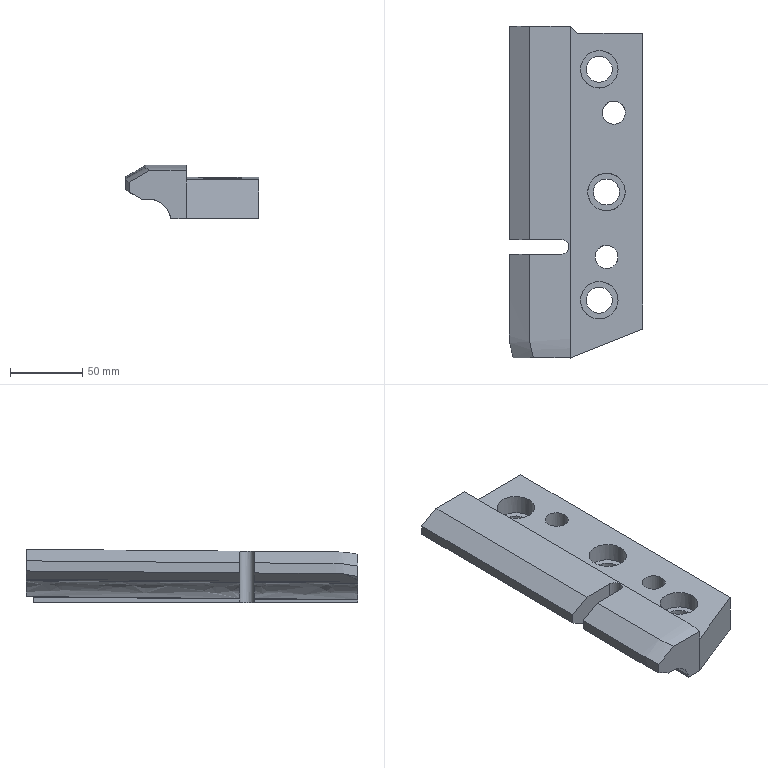Part | NX | features solid 2 | 1 solid | 46 faces | box 92.255 x 230 x 36.978 mm | volume 481393 mm3 | spline 23 | plane 14 | cylinder 9 | commonest cylinder face diameters 18 x3 26 x3 16 x2 10 x1